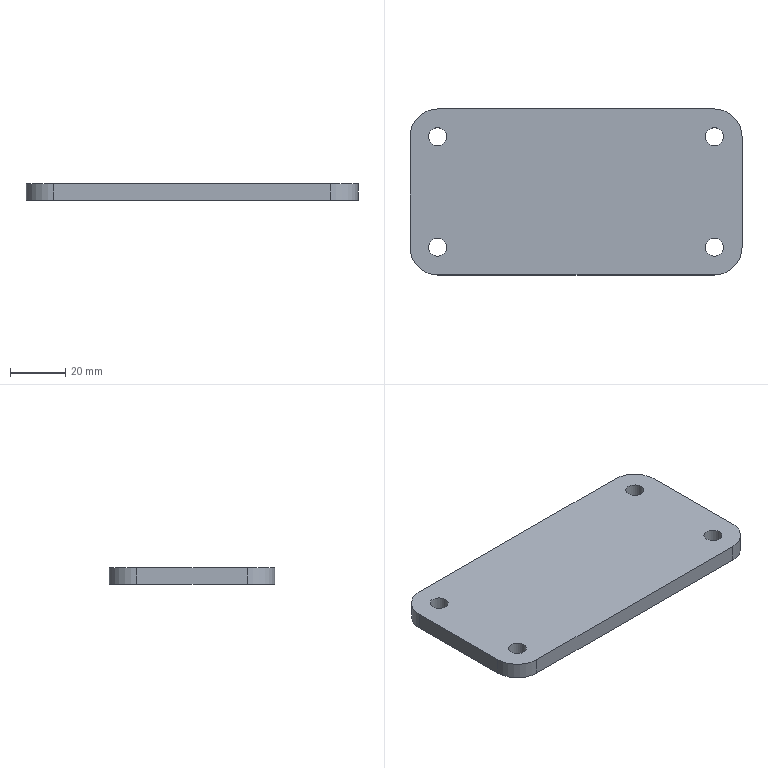Part | STEP file | JBJ-P-1015-01 | 1 solid | 14 faces | box 120 x 60 x 6 mm | volume 41889 mm3 | cylinder 8 | plane 6 | commonest cylinder face diameters 6.5 x4 20 x4
STEP:
#1=CARTESIAN_POINT('',(0.,-10.,0.));
#2=VERTEX_POINT('',#1);
#3=CARTESIAN_POINT('',(0.,-50.,0.));
#4=VERTEX_POINT('',#3);
#5=CARTESIAN_POINT('',(0.,0.,0.));
#6=DIRECTION('',(0.,-1.,0.));
#7=VECTOR('',#6,1000.);
#8=LINE('',#5,#7);
#9=EDGE_CURVE('',#2,#4,#8,.T.);
#10=ORIENTED_EDGE('',*,*,#9,.T.);
#11=CARTESIAN_POINT('',(0.,-50.,6.));
#12=VERTEX_POINT('',#11);
#13=CARTESIAN_POINT('',(0.,-50.,6.));
#14=DIRECTION('',(0.,0.,1.));
#15=VECTOR('',#14,1000.);
#16=LINE('',#13,#15);
#17=EDGE_CURVE('',#4,#12,#16,.T.);
#18=ORIENTED_EDGE('',*,*,#17,.T.);
#19=CARTESIAN_POINT('',(0.,-10.,6.));
#20=VERTEX_POINT('',#19);
#21=CARTESIAN_POINT('',(0.,0.,6.));
#22=DIRECTION('',(0.,-1.,0.));
#23=VECTOR('',#22,1000.);
#24=LINE('',#21,#23);
#25=EDGE_CURVE('',#20,#12,#24,.T.);
#26=ORIENTED_EDGE('',*,*,#25,.F.);
#27=CARTESIAN_POINT('',(0.,-10.,6.));
#28=DIRECTION('',(0.,0.,-1.));
#29=VECTOR('',#28,1000.);
#30=LINE('',#27,#29);
#31=EDGE_CURVE('',#20,#2,#30,.T.);
#32=ORIENTED_EDGE('',*,*,#31,.T.);
#33=EDGE_LOOP('',(#10,#18,#26,#32));
#34=FACE_OUTER_BOUND('',#33,.T.);
#35=CARTESIAN_POINT('',(0.,0.,6.));
#36=DIRECTION('',(1.,0.,0.));
#37=DIRECTION('',(0.,0.,-1.));
#38=AXIS2_PLACEMENT_3D('',#35,#36,#37);
#39=PLANE('',#38);
#40=ADVANCED_FACE('',(#34),#39,.F.);
#41=CARTESIAN_POINT('',(10.,-60.,0.));
#42=VERTEX_POINT('',#41);
#43=CARTESIAN_POINT('',(110.,-60.,0.));
#44=VERTEX_POINT('',#43);
#45=CARTESIAN_POINT('',(0.,-60.,0.));
#46=DIRECTION('',(1.,0.,0.));
#47=VECTOR('',#46,1000.);
#48=LINE('',#45,#47);
#49=EDGE_CURVE('',#42,#44,#48,.T.);
#50=ORIENTED_EDGE('',*,*,#49,.T.);
#51=CARTESIAN_POINT('',(110.,-60.,6.));
#52=VERTEX_POINT('',#51);
#53=CARTESIAN_POINT('',(110.,-60.,6.));
#54=DIRECTION('',(0.,0.,1.));
#55=VECTOR('',#54,1000.);
#56=LINE('',#53,#55);
#57=EDGE_CURVE('',#44,#52,#56,.T.);
#58=ORIENTED_EDGE('',*,*,#57,.T.);
#59=CARTESIAN_POINT('',(10.,-60.,6.));
#60=VERTEX_POINT('',#59);
#61=CARTESIAN_POINT('',(0.,-60.,6.));
#62=DIRECTION('',(1.,0.,0.));
#63=VECTOR('',#62,1000.);
#64=LINE('',#61,#63);
#65=EDGE_CURVE('',#60,#52,#64,.T.);
#66=ORIENTED_EDGE('',*,*,#65,.F.);
#67=CARTESIAN_POINT('',(10.,-60.,6.));
#68=DIRECTION('',(0.,0.,-1.));
#69=VECTOR('',#68,1000.);
#70=LINE('',#67,#69);
#71=EDGE_CURVE('',#60,#42,#70,.T.);
#72=ORIENTED_EDGE('',*,*,#71,.T.);
#73=EDGE_LOOP('',(#50,#58,#66,#72));
#74=FACE_OUTER_BOUND('',#73,.T.);
#75=CARTESIAN_POINT('',(0.,-60.,6.));
#76=DIRECTION('',(0.,1.,0.));
#77=DIRECTION('',(0.,0.,1.));
#78=AXIS2_PLACEMENT_3D('',#75,#76,#77);
#79=PLANE('',#78);
#80=ADVANCED_FACE('',(#74),#79,.F.);
#81=CARTESIAN_POINT('',(120.,-50.,0.));
#82=VERTEX_POINT('',#81);
#83=CARTESIAN_POINT('',(120.,-10.,0.));
#84=VERTEX_POINT('',#83);
#85=CARTESIAN_POINT('',(120.,0.,0.));
#86=DIRECTION('',(0.,1.,0.));
#87=VECTOR('',#86,1000.);
#88=LINE('',#85,#87);
#89=EDGE_CURVE('',#82,#84,#88,.T.);
#90=ORIENTED_EDGE('',*,*,#89,.T.);
#91=CARTESIAN_POINT('',(120.,-10.,6.));
#92=VERTEX_POINT('',#91);
#93=CARTESIAN_POINT('',(120.,-10.,6.));
#94=DIRECTION('',(0.,0.,1.));
#95=VECTOR('',#94,1000.);
#96=LINE('',#93,#95);
#97=EDGE_CURVE('',#84,#92,#96,.T.);
#98=ORIENTED_EDGE('',*,*,#97,.T.);
#99=CARTESIAN_POINT('',(120.,-50.,6.));
#100=VERTEX_POINT('',#99);
#101=CARTESIAN_POINT('',(120.,0.,6.));
#102=DIRECTION('',(0.,1.,0.));
#103=VECTOR('',#102,1000.);
#104=LINE('',#101,#103);
#105=EDGE_CURVE('',#100,#92,#104,.T.);
#106=ORIENTED_EDGE('',*,*,#105,.F.);
#107=CARTESIAN_POINT('',(120.,-50.,6.));
#108=DIRECTION('',(0.,0.,-1.));
#109=VECTOR('',#108,1000.);
#110=LINE('',#107,#109);
#111=EDGE_CURVE('',#100,#82,#110,.T.);
#112=ORIENTED_EDGE('',*,*,#111,.T.);
#113=EDGE_LOOP('',(#90,#98,#106,#112));
#114=FACE_OUTER_BOUND('',#113,.T.);
#115=CARTESIAN_POINT('',(120.,0.,6.));
#116=DIRECTION('',(-1.,0.,0.));
#117=DIRECTION('',(0.,-1.,0.));
#118=AXIS2_PLACEMENT_3D('',#115,#116,#117);
#119=PLANE('',#118);
#120=ADVANCED_FACE('',(#114),#119,.F.);
#121=CARTESIAN_POINT('',(110.,0.,6.));
#122=VERTEX_POINT('',#121);
#123=CARTESIAN_POINT('',(10.,0.,6.));
#124=VERTEX_POINT('',#123);
#125=CARTESIAN_POINT('',(0.,0.,6.));
#126=DIRECTION('',(-1.,0.,0.));
#127=VECTOR('',#126,1000.);
#128=LINE('',#125,#127);
#129=EDGE_CURVE('',#122,#124,#128,.T.);
#130=ORIENTED_EDGE('',*,*,#129,.F.);
#131=CARTESIAN_POINT('',(110.,0.,0.));
#132=VERTEX_POINT('',#131);
#133=CARTESIAN_POINT('',(110.,0.,6.));
#134=DIRECTION('',(0.,0.,-1.));
#135=VECTOR('',#134,1000.);
#136=LINE('',#133,#135);
#137=EDGE_CURVE('',#122,#132,#136,.T.);
#138=ORIENTED_EDGE('',*,*,#137,.T.);
#139=CARTESIAN_POINT('',(10.,0.,0.));
#140=VERTEX_POINT('',#139);
#141=CARTESIAN_POINT('',(0.,0.,0.));
#142=DIRECTION('',(-1.,0.,0.));
#143=VECTOR('',#142,1000.);
#144=LINE('',#141,#143);
#145=EDGE_CURVE('',#132,#140,#144,.T.);
#146=ORIENTED_EDGE('',*,*,#145,.T.);
#147=CARTESIAN_POINT('',(10.,0.,6.));
#148=DIRECTION('',(0.,0.,1.));
#149=VECTOR('',#148,1000.);
#150=LINE('',#147,#149);
#151=EDGE_CURVE('',#140,#124,#150,.T.);
#152=ORIENTED_EDGE('',*,*,#151,.T.);
#153=EDGE_LOOP('',(#130,#138,#146,#152));
#154=FACE_OUTER_BOUND('',#153,.T.);
#155=CARTESIAN_POINT('',(0.,0.,6.));
#156=DIRECTION('',(0.,-1.,0.));
#157=DIRECTION('',(0.,0.,-1.));
#158=AXIS2_PLACEMENT_3D('',#155,#156,#157);
#159=PLANE('',#158);
#160=ADVANCED_FACE('',(#154),#159,.F.);
#161=CARTESIAN_POINT('',(13.25,-10.,6.));
#162=VERTEX_POINT('',#161);
#163=CARTESIAN_POINT('',(10.,-10.,6.));
#164=DIRECTION('',(0.,0.,1.));
#165=DIRECTION('',(1.,0.,0.));
#166=AXIS2_PLACEMENT_3D('',#163,#164,#165);
#167=CIRCLE('',#166,3.25);
#168=EDGE_CURVE('',#162,#162,#167,.T.);
#169=ORIENTED_EDGE('',*,*,#168,.F.);
#170=EDGE_LOOP('',(#169));
#171=FACE_BOUND('',#170,.T.);
#172=CARTESIAN_POINT('',(13.25,-50.,6.));
#173=VERTEX_POINT('',#172);
#174=CARTESIAN_POINT('',(10.,-50.,6.));
#175=DIRECTION('',(0.,0.,1.));
#176=DIRECTION('',(1.,0.,0.));
#177=AXIS2_PLACEMENT_3D('',#174,#175,#176);
#178=CIRCLE('',#177,3.25);
#179=EDGE_CURVE('',#173,#173,#178,.T.);
#180=ORIENTED_EDGE('',*,*,#179,.F.);
#181=EDGE_LOOP('',(#180));
#182=FACE_BOUND('',#181,.T.);
#183=CARTESIAN_POINT('',(113.25,-50.,6.));
#184=VERTEX_POINT('',#183);
#185=CARTESIAN_POINT('',(110.,-50.,6.));
#186=DIRECTION('',(0.,0.,1.));
#187=DIRECTION('',(1.,0.,0.));
#188=AXIS2_PLACEMENT_3D('',#185,#186,#187);
#189=CIRCLE('',#188,3.25);
#190=EDGE_CURVE('',#184,#184,#189,.T.);
#191=ORIENTED_EDGE('',*,*,#190,.F.);
#192=EDGE_LOOP('',(#191));
#193=FACE_BOUND('',#192,.T.);
#194=CARTESIAN_POINT('',(113.25,-10.,6.));
#195=VERTEX_POINT('',#194);
#196=CARTESIAN_POINT('',(110.,-10.,6.));
#197=DIRECTION('',(0.,0.,1.));
#198=DIRECTION('',(1.,0.,0.));
#199=AXIS2_PLACEMENT_3D('',#196,#197,#198);
#200=CIRCLE('',#199,3.25);
#201=EDGE_CURVE('',#195,#195,#200,.T.);
#202=ORIENTED_EDGE('',*,*,#201,.F.);
#203=EDGE_LOOP('',(#202));
#204=FACE_BOUND('',#203,.T.);
#205=ORIENTED_EDGE('',*,*,#105,.T.);
#206=CARTESIAN_POINT('',(110.,-10.,6.));
#207=DIRECTION('',(0.,0.,1.));
#208=DIRECTION('',(1.,0.,0.));
#209=AXIS2_PLACEMENT_3D('',#206,#207,#208);
#210=CIRCLE('',#209,10.);
#211=EDGE_CURVE('',#92,#122,#210,.T.);
#212=ORIENTED_EDGE('',*,*,#211,.T.);
#213=ORIENTED_EDGE('',*,*,#129,.T.);
#214=CARTESIAN_POINT('',(10.,-10.,6.));
#215=DIRECTION('',(0.,0.,1.));
#216=DIRECTION('',(1.,0.,0.));
#217=AXIS2_PLACEMENT_3D('',#214,#215,#216);
#218=CIRCLE('',#217,10.);
#219=EDGE_CURVE('',#124,#20,#218,.T.);
#220=ORIENTED_EDGE('',*,*,#219,.T.);
#221=ORIENTED_EDGE('',*,*,#25,.T.);
#222=CARTESIAN_POINT('',(10.,-50.,6.));
#223=DIRECTION('',(0.,0.,1.));
#224=DIRECTION('',(1.,0.,0.));
#225=AXIS2_PLACEMENT_3D('',#222,#223,#224);
#226=CIRCLE('',#225,10.);
#227=EDGE_CURVE('',#12,#60,#226,.T.);
#228=ORIENTED_EDGE('',*,*,#227,.T.);
#229=ORIENTED_EDGE('',*,*,#65,.T.);
#230=CARTESIAN_POINT('',(110.,-50.,6.));
#231=DIRECTION('',(0.,0.,1.));
#232=DIRECTION('',(1.,0.,0.));
#233=AXIS2_PLACEMENT_3D('',#230,#231,#232);
#234=CIRCLE('',#233,10.);
#235=EDGE_CURVE('',#52,#100,#234,.T.);
#236=ORIENTED_EDGE('',*,*,#235,.T.);
#237=EDGE_LOOP('',(#205,#212,#213,#220,#221,#228,#229,#236));
#238=FACE_OUTER_BOUND('',#237,.T.);
#239=CARTESIAN_POINT('',(0.,0.,6.));
#240=DIRECTION('',(0.,0.,1.));
#241=DIRECTION('',(1.,0.,0.));
#242=AXIS2_PLACEMENT_3D('',#239,#240,#241);
#243=PLANE('',#242);
#244=ADVANCED_FACE('',(#171,#182,#193,#204,#238),#243,.T.);
#245=CARTESIAN_POINT('',(13.25,-10.,0.));
#246=VERTEX_POINT('',#245);
#247=CARTESIAN_POINT('',(10.,-10.,0.));
#248=DIRECTION('',(0.,0.,1.));
#249=DIRECTION('',(1.,0.,0.));
#250=AXIS2_PLACEMENT_3D('',#247,#248,#249);
#251=CIRCLE('',#250,3.25);
#252=EDGE_CURVE('',#246,#246,#251,.T.);
#253=ORIENTED_EDGE('',*,*,#252,.T.);
#254=EDGE_LOOP('',(#253));
#255=FACE_BOUND('',#254,.T.);
#256=CARTESIAN_POINT('',(13.25,-50.,0.));
#257=VERTEX_POINT('',#256);
#258=CARTESIAN_POINT('',(10.,-50.,0.));
#259=DIRECTION('',(0.,0.,1.));
#260=DIRECTION('',(1.,0.,0.));
#261=AXIS2_PLACEMENT_3D('',#258,#259,#260);
#262=CIRCLE('',#261,3.25);
#263=EDGE_CURVE('',#257,#257,#262,.T.);
#264=ORIENTED_EDGE('',*,*,#263,.T.);
#265=EDGE_LOOP('',(#264));
#266=FACE_BOUND('',#265,.T.);
#267=CARTESIAN_POINT('',(113.25,-50.,0.));
#268=VERTEX_POINT('',#267);
#269=CARTESIAN_POINT('',(110.,-50.,0.));
#270=DIRECTION('',(0.,0.,1.));
#271=DIRECTION('',(1.,0.,0.));
#272=AXIS2_PLACEMENT_3D('',#269,#270,#271);
#273=CIRCLE('',#272,3.25);
#274=EDGE_CURVE('',#268,#268,#273,.T.);
#275=ORIENTED_EDGE('',*,*,#274,.T.);
#276=EDGE_LOOP('',(#275));
#277=FACE_BOUND('',#276,.T.);
#278=CARTESIAN_POINT('',(113.25,-10.,0.));
#279=VERTEX_POINT('',#278);
#280=CARTESIAN_POINT('',(110.,-10.,0.));
#281=DIRECTION('',(0.,0.,1.));
#282=DIRECTION('',(1.,0.,0.));
#283=AXIS2_PLACEMENT_3D('',#280,#281,#282);
#284=CIRCLE('',#283,3.25);
#285=EDGE_CURVE('',#279,#279,#284,.T.);
#286=ORIENTED_EDGE('',*,*,#285,.T.);
#287=EDGE_LOOP('',(#286));
#288=FACE_BOUND('',#287,.T.);
#289=ORIENTED_EDGE('',*,*,#145,.F.);
#290=CARTESIAN_POINT('',(110.,-10.,0.));
#291=DIRECTION('',(0.,0.,-1.));
#292=DIRECTION('',(1.,0.,0.));
#293=AXIS2_PLACEMENT_3D('',#290,#291,#292);
#294=CIRCLE('',#293,10.);
#295=EDGE_CURVE('',#132,#84,#294,.T.);
#296=ORIENTED_EDGE('',*,*,#295,.T.);
#297=ORIENTED_EDGE('',*,*,#89,.F.);
#298=CARTESIAN_POINT('',(110.,-50.,0.));
#299=DIRECTION('',(0.,0.,-1.));
#300=DIRECTION('',(1.,0.,0.));
#301=AXIS2_PLACEMENT_3D('',#298,#299,#300);
#302=CIRCLE('',#301,10.);
#303=EDGE_CURVE('',#82,#44,#302,.T.);
#304=ORIENTED_EDGE('',*,*,#303,.T.);
#305=ORIENTED_EDGE('',*,*,#49,.F.);
#306=CARTESIAN_POINT('',(10.,-50.,0.));
#307=DIRECTION('',(0.,0.,-1.));
#308=DIRECTION('',(1.,0.,0.));
#309=AXIS2_PLACEMENT_3D('',#306,#307,#308);
#310=CIRCLE('',#309,10.);
#311=EDGE_CURVE('',#42,#4,#310,.T.);
#312=ORIENTED_EDGE('',*,*,#311,.T.);
#313=ORIENTED_EDGE('',*,*,#9,.F.);
#314=CARTESIAN_POINT('',(10.,-10.,0.));
#315=DIRECTION('',(0.,0.,-1.));
#316=DIRECTION('',(1.,0.,0.));
#317=AXIS2_PLACEMENT_3D('',#314,#315,#316);
#318=CIRCLE('',#317,10.);
#319=EDGE_CURVE('',#2,#140,#318,.T.);
#320=ORIENTED_EDGE('',*,*,#319,.T.);
#321=EDGE_LOOP('',(#289,#296,#297,#304,#305,#312,#313,#320));
#322=FACE_OUTER_BOUND('',#321,.T.);
#323=CARTESIAN_POINT('',(0.,0.,0.));
#324=DIRECTION('',(0.,0.,1.));
#325=DIRECTION('',(1.,0.,0.));
#326=AXIS2_PLACEMENT_3D('',#323,#324,#325);
#327=PLANE('',#326);
#328=ADVANCED_FACE('',(#255,#266,#277,#288,#322),#327,.F.);
#329=ORIENTED_EDGE('',*,*,#285,.F.);
#330=EDGE_LOOP('',(#329));
#331=FACE_OUTER_BOUND('',#330,.T.);
#332=ORIENTED_EDGE('',*,*,#201,.T.);
#333=EDGE_LOOP('',(#332));
#334=FACE_OUTER_BOUND('',#333,.T.);
#335=CARTESIAN_POINT('',(110.,-10.,6.));
#336=DIRECTION('',(0.,0.,1.));
#337=DIRECTION('',(1.,0.,0.));
#338=AXIS2_PLACEMENT_3D('',#335,#336,#337);
#339=CYLINDRICAL_SURFACE('',#338,3.25);
#340=ADVANCED_FACE('',(#331,#334),#339,.F.);
#341=ORIENTED_EDGE('',*,*,#274,.F.);
#342=EDGE_LOOP('',(#341));
#343=FACE_OUTER_BOUND('',#342,.T.);
#344=ORIENTED_EDGE('',*,*,#190,.T.);
#345=EDGE_LOOP('',(#344));
#346=FACE_OUTER_BOUND('',#345,.T.);
#347=CARTESIAN_POINT('',(110.,-50.,6.));
#348=DIRECTION('',(0.,0.,1.));
#349=DIRECTION('',(1.,0.,0.));
#350=AXIS2_PLACEMENT_3D('',#347,#348,#349);
#351=CYLINDRICAL_SURFACE('',#350,3.25);
#352=ADVANCED_FACE('',(#343,#346),#351,.F.);
#353=ORIENTED_EDGE('',*,*,#263,.F.);
#354=EDGE_LOOP('',(#353));
#355=FACE_OUTER_BOUND('',#354,.T.);
#356=ORIENTED_EDGE('',*,*,#179,.T.);
#357=EDGE_LOOP('',(#356));
#358=FACE_OUTER_BOUND('',#357,.T.);
#359=CARTESIAN_POINT('',(10.,-50.,6.));
#360=DIRECTION('',(0.,0.,1.));
#361=DIRECTION('',(1.,0.,0.));
#362=AXIS2_PLACEMENT_3D('',#359,#360,#361);
#363=CYLINDRICAL_SURFACE('',#362,3.25);
#364=ADVANCED_FACE('',(#355,#358),#363,.F.);
#365=ORIENTED_EDGE('',*,*,#252,.F.);
#366=EDGE_LOOP('',(#365));
#367=FACE_OUTER_BOUND('',#366,.T.);
#368=ORIENTED_EDGE('',*,*,#168,.T.);
#369=EDGE_LOOP('',(#368));
#370=FACE_OUTER_BOUND('',#369,.T.);
#371=CARTESIAN_POINT('',(10.,-10.,6.));
#372=DIRECTION('',(0.,0.,1.));
#373=DIRECTION('',(1.,0.,0.));
#374=AXIS2_PLACEMENT_3D('',#371,#372,#373);
#375=CYLINDRICAL_SURFACE('',#374,3.25);
#376=ADVANCED_FACE('',(#367,#370),#375,.F.);
#377=ORIENTED_EDGE('',*,*,#211,.F.);
#378=ORIENTED_EDGE('',*,*,#97,.F.);
#379=ORIENTED_EDGE('',*,*,#295,.F.);
#380=ORIENTED_EDGE('',*,*,#137,.F.);
#381=EDGE_LOOP('',(#377,#378,#379,#380));
#382=FACE_OUTER_BOUND('',#381,.T.);
#383=CARTESIAN_POINT('',(110.,-10.,6.));
#384=DIRECTION('',(0.,0.,-1.));
#385=DIRECTION('',(-1.,0.,0.));
#386=AXIS2_PLACEMENT_3D('',#383,#384,#385);
#387=CYLINDRICAL_SURFACE('',#386,10.);
#388=ADVANCED_FACE('',(#382),#387,.T.);
#389=ORIENTED_EDGE('',*,*,#235,.F.);
#390=ORIENTED_EDGE('',*,*,#57,.F.);
#391=ORIENTED_EDGE('',*,*,#303,.F.);
#392=ORIENTED_EDGE('',*,*,#111,.F.);
#393=EDGE_LOOP('',(#389,#390,#391,#392));
#394=FACE_OUTER_BOUND('',#393,.T.);
#395=CARTESIAN_POINT('',(110.,-50.,6.));
#396=DIRECTION('',(0.,0.,-1.));
#397=DIRECTION('',(-1.,0.,0.));
#398=AXIS2_PLACEMENT_3D('',#395,#396,#397);
#399=CYLINDRICAL_SURFACE('',#398,10.);
#400=ADVANCED_FACE('',(#394),#399,.T.);
#401=ORIENTED_EDGE('',*,*,#227,.F.);
#402=ORIENTED_EDGE('',*,*,#17,.F.);
#403=ORIENTED_EDGE('',*,*,#311,.F.);
#404=ORIENTED_EDGE('',*,*,#71,.F.);
#405=EDGE_LOOP('',(#401,#402,#403,#404));
#406=FACE_OUTER_BOUND('',#405,.T.);
#407=CARTESIAN_POINT('',(10.,-50.,6.));
#408=DIRECTION('',(0.,0.,-1.));
#409=DIRECTION('',(-1.,0.,0.));
#410=AXIS2_PLACEMENT_3D('',#407,#408,#409);
#411=CYLINDRICAL_SURFACE('',#410,10.);
#412=ADVANCED_FACE('',(#406),#411,.T.);
#413=ORIENTED_EDGE('',*,*,#219,.F.);
#414=ORIENTED_EDGE('',*,*,#151,.F.);
#415=ORIENTED_EDGE('',*,*,#319,.F.);
#416=ORIENTED_EDGE('',*,*,#31,.F.);
#417=EDGE_LOOP('',(#413,#414,#415,#416));
#418=FACE_OUTER_BOUND('',#417,.T.);
#419=CARTESIAN_POINT('',(10.,-10.,6.));
#420=DIRECTION('',(0.,0.,-1.));
#421=DIRECTION('',(-1.,0.,0.));
#422=AXIS2_PLACEMENT_3D('',#419,#420,#421);
#423=CYLINDRICAL_SURFACE('',#422,10.);
#424=ADVANCED_FACE('',(#418),#423,.T.);
#425=CLOSED_SHELL('',(#40,#80,#120,#160,#244,#328,#340,#352,#364,#376,#388,#400,#412,#424));
#426=MANIFOLD_SOLID_BREP('',#425);
#427=CARTESIAN_POINT('',(0.,0.,0.));
#428=DIRECTION('',(0.,0.,1.));
#429=DIRECTION('',(1.,0.,0.));
#430=AXIS2_PLACEMENT_3D('',#427,#428,#429);
#431=(LENGTH_UNIT()NAMED_UNIT(*)SI_UNIT(.MILLI.,.METRE.));
#432=UNCERTAINTY_MEASURE_WITH_UNIT(LENGTH_MEASURE(0.00001),#431,'','');
#433=(NAMED_UNIT(*)PLANE_ANGLE_UNIT()SI_UNIT($,.RADIAN.));
#434=(NAMED_UNIT(*)SI_UNIT($,.STERADIAN.)SOLID_ANGLE_UNIT());
#435=(GEOMETRIC_REPRESENTATION_CONTEXT(3)GLOBAL_UNCERTAINTY_ASSIGNED_CONTEXT((#432))GLOBAL_UNIT_ASSIGNED_CONTEXT((#431,#433,#434))REPRESENTATION_CONTEXT('',''));
#436=ADVANCED_BREP_SHAPE_REPRESENTATION('',(#426,#430),#435);